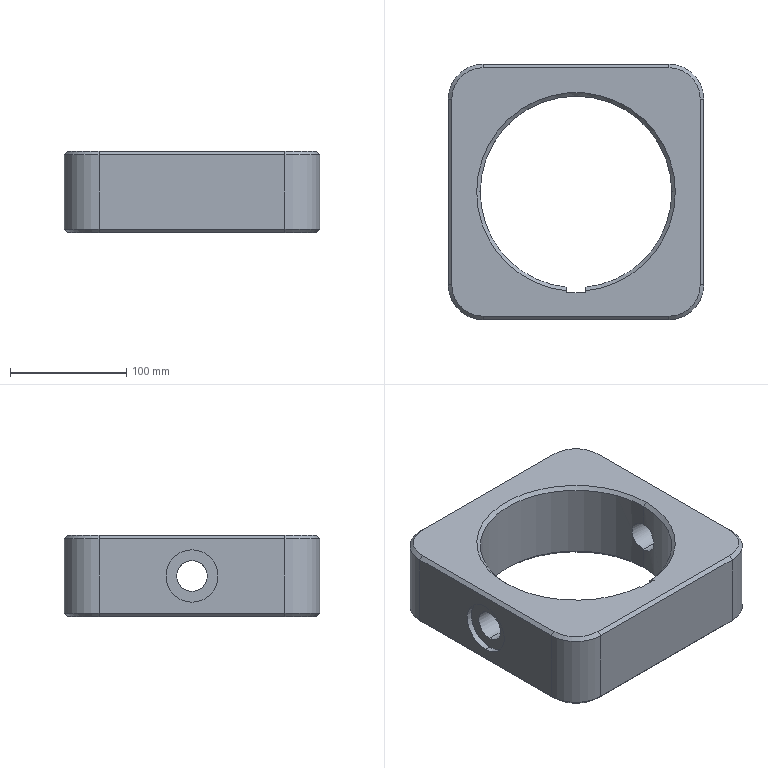Part | SolidWorks | features ICE 3, Chamfer 1, Extrusion 1, Fillet 1, HoleWzd 1, MirrorPattern 1 | 1 solid | 48 faces | box 220 x 220 x 70 mm | volume 1778957 mm3 | plane 19 | cylinder 15 | cone 14 | commonest cylinder face diameters 26.5 x4 45 x4 60 x4 165 x3